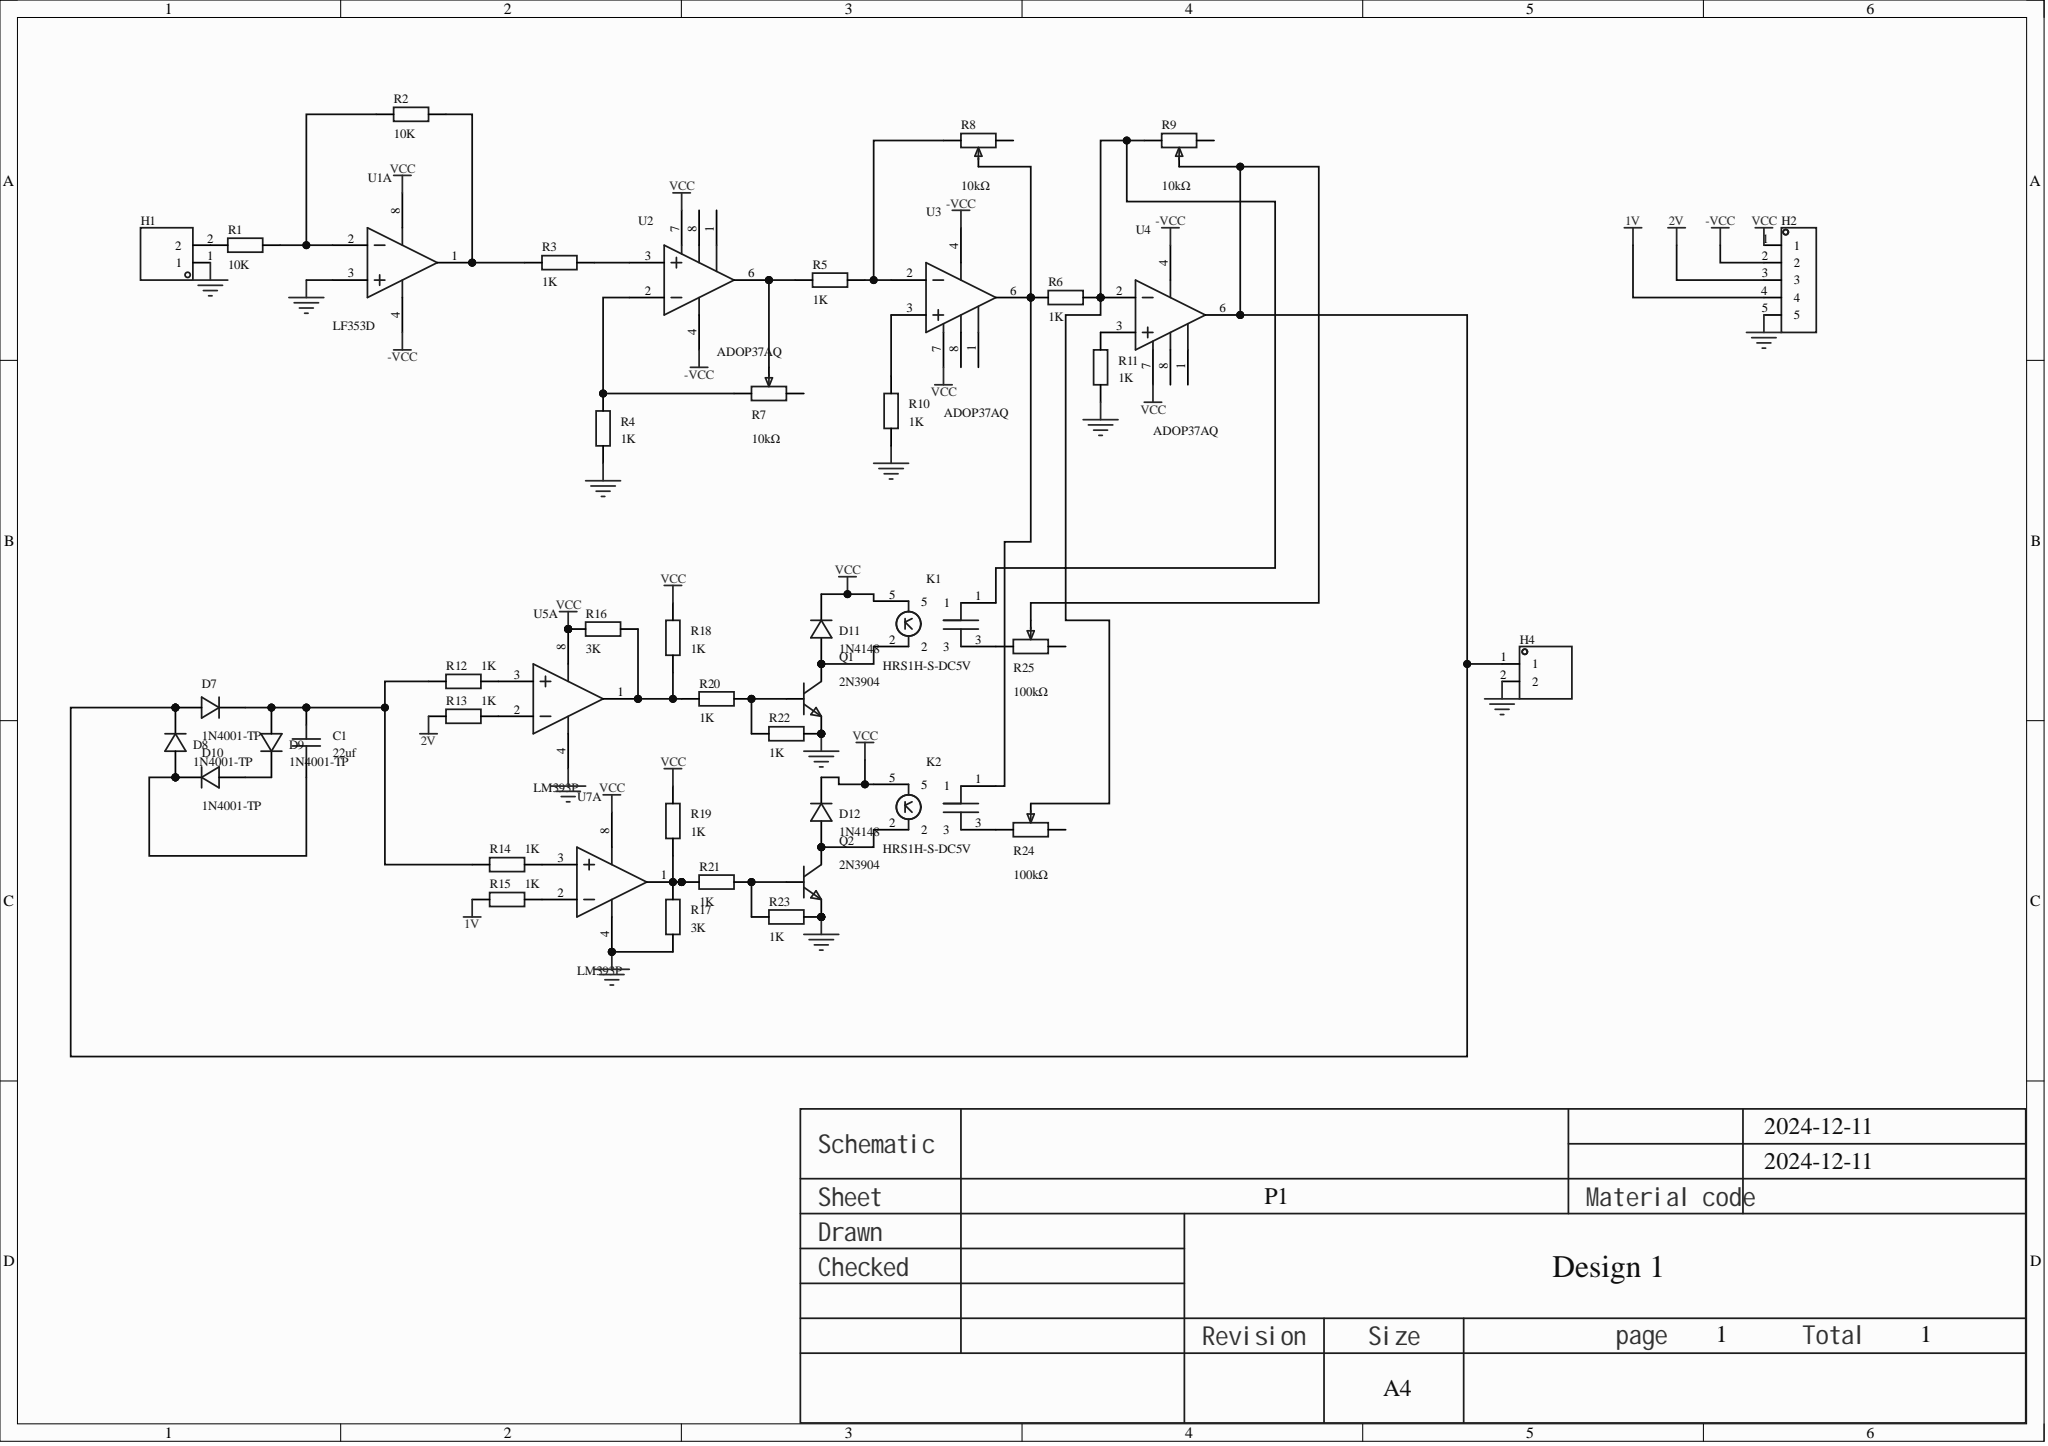Circuit board | Altium Designer | 45 parts | 32 nets
Bill of materials:
Comment,Description,Designator,Footprint,LibRef,Quantity
"22uf","","C1","C0805","CAP_0805","1"
"1N4001-TP","","D7, D8, D9, D10","DO-41_BD2.4-L4.7-P8.70-D0.9-RD","1N4001-TP","4"
"1N4148","Diode configuration: -; forward voltage (Vf): 1.1V@1A; DC reverse withstand voltage (Vr): 50V; rectified current: 1A;","D11, D12","DO-41_BD2.4-L4.7-P8.70-D0.9-RD","1N4001_C2456","2"
"","","H1, H4","HDR-TH_2P-P2.54-V-M-1","HDR-M_2.54_1x2P","2"
"","","H2","HDR-TH_5P-P2.54-V-M","HDR-M_2.54_1x5P","1"
"HRS1H-S-DC5V","Ultra-miniature relay 15.6x10.6x11.8 (mm), 3A contact switching capacity, single-pole changeover, high sensitivity","K1, K2","RELAY-TH_HRS1H-S-DC3V","HRS1H-S-DC5V","2"
"2N3904","Transistor type: NPN; collector current (Ic): 200mA; collector-emitter breakdown voltage (Vceo): 40V; power (Pd): 625mW; DC current gain (hFE@Ic,Vce): 60@50mA,1V;","Q1, Q2","TO-92-3_L4.9-W3.7-P1.27-L","2N3904","2"
"10K","","R1, R2","R0603","Res_0603","2"
"1K","","R3, R4, R5, R6, R10, R11, R12, R13, R14, R15, R18, R19, R20, R21, R22, R23","R0603","Res_0603","16"
"10kΩ","","R7, R8, R9","R_3296","R_3296","3"
"3K","","R16, R17","R0603","Res_0603","2"
"100kΩ","","R24, R25","R_3296","R_3296","2"
"LF353D","GBP: 3MHz; input bias current (Ib): 50pA; input offset voltage (Vos): 5mV; slew rate (SR): 13V/us;","U1","SOIC-8_L4.9-W3.9-P1.27-LS6.0-BL","LF353D","1"
"ADOP37AQ","Number of amplifiers: single; input bias current (Ib): 10nA; input offset voltage (Vos): 10uV; GBP: 63MHz; slew rate (SR): 17V/us; bandwidth (-3db): -;","U2, U3, U4","PDIP-8_L9.6-W6.4-P2.54-LS7.6-BL","ADOP37AQ","3"
"LM393P","Input offset voltage (Vos): 5mV; input bias current (Ib): 250nA;","U5, U7","DIP-8_L10.1-W6.3-P2.54-LS7.6-BL-1","LM393P","2"
Netlist (Protel format):
[
C1
C0805
22uf



]
[
D7
DO-41_BD2.4-L4.7-P8.70-D0.9-RD
1N4001-TP



]
[
D8
DO-41_BD2.4-L4.7-P8.70-D0.9-RD
1N4001-TP



]
[
D9
DO-41_BD2.4-L4.7-P8.70-D0.9-RD
1N4001-TP



]
[
D10
DO-41_BD2.4-L4.7-P8.70-D0.9-RD
1N4001-TP



]
[
D11
DO-41_BD2.4-L4.7-P8.70-D0.9-RD
1N4148



]
[
D12
DO-41_BD2.4-L4.7-P8.70-D0.9-RD
1N4148



]
[
H1
HDR-TH_2P-P2.54-V-M-1




]
[
H2
HDR-TH_5P-P2.54-V-M




]
[
H4
HDR-TH_2P-P2.54-V-M-1




]
[
K1
RELAY-TH_HRS1H-S-DC3V
HRS1H-S-DC5V



]
[
K2
RELAY-TH_HRS1H-S-DC3V
HRS1H-S-DC5V



]
[
Q1
TO-92-3_L4.9-W3.7-P1.27-L
2N3904



]
[
Q2
TO-92-3_L4.9-W3.7-P1.27-L
2N3904



]
[
R1
R0603
10K



]
[
R2
R0603
10K



]
[
R3
R0603
1K



]
[
R4
R0603
1K



]
[
R5
R0603
1K



]
[
R6
R0603
1K



]
[
R7
R_3296
10kΩ



]
[
R8
R_3296
10kΩ



]
[
R9
R_3296
10kΩ



]
[
R10
R0603
1K



]
[
R11
R0603
1K



]
[
R12
R0603
1K



]
[
R13
R0603
1K



]
[
R14
R0603
1K



]
[
R15
R0603
1K



]
[
R16
R0603
3K



]
[
R17
R0603
3K



]
[
R18
R0603
1K



]
[
R19
R0603
1K



]
[
R20
R0603
1K



]
[
R21
R0603
1K



]
[
R22
R0603
1K



]
[
R23
R0603
1K



]
[
R24
R_3296
100kΩ



]
[
R25
R_3296
100kΩ



]
[
U1
SOIC-8_L4.9-W3.9-P1.27-LS6.0-BL
LF353D



]
[
U2
PDIP-8_L9.6-W6.4-P2.54-LS7.6-BL
ADOP37AQ



]
[
U3
PDIP-8_L9.6-W6.4-P2.54-LS7.6-BL
ADOP37AQ



]
[
U4
PDIP-8_L9.6-W6.4-P2.54-LS7.6-BL
ADOP37AQ



]
[
U5
DIP-8_L10.1-W6.3-P2.54-LS7.6-BL-1
LM393P



]
[
U7
DIP-8_L10.1-W6.3-P2.54-LS7.6-BL-1
LM393P



]
(
VCC
D11-1
D12-1
H2-1
K1-5
K2-5
R16-1
R18-2
R19-2
U1-8
U2-7
U3-7
U4-7
U5-8
U7-8
)
(
NetR17_2
R17-2
R19-1
R21-1
U7-1
)
(
NetR16_2
R16-2
R18-1
R20-1
U5-1
)
(
NetR15_2
R15-2
U7-2
)
(
NetR14_2
R14-2
U7-3
)
(
NetR13_2
R13-2
U5-2
)
(
NetR12_2
R12-2
U5-3
)
(
NetR11_2
R11-2
U4-3
)
(
NetR10_2
R10-2
U3-3
)
(
NetR5_2
R5-2
R8-1
U3-2
)
(
NetR5_1
R5-1
R7-2
U2-6
)
(
NetR4_2
R4-2
R7-3
U2-2
)
(
NetR3_2
R3-2
U2-3
)
(
NetR2_2
R2-2
R3-1
U1-1
)
(
NetR1_2
R1-2
R2-1
U1-2
)
(
NetQ2_2
Q2-2
R21-2
R23-1
)
(
NetQ1_2
Q1-2
R20-2
R22-1
)
(
NetK2_3
K2-3
R24-3
)
(
NetK2_1
K2-1
R6-1
R8-2
U3-6
)
(
NetK1_3
K1-3
R25-3
)
(
NetK1_1
K1-1
R6-2
R9-1
R24-2
U4-2
)
(
NetH1_2
H1-2
R1-1
)
(
NetD12_2
D12-2
K2-2
Q2-3
)
(
NetD11_2
D11-2
K1-2
Q1-3
)
(
NetD9_1
D9-1
D10-2
)
(
NetD7_2
D7-2
D8-1
H4-1
R9-2
R25-2
U4-6
)
(
NetC1_2
C1-2
D7-1
D9-2
R12-1
R14-1
)
(
NetC1_1
C1-1
D8-2
D10-1
)
(
GND
H1-1
H2-5
H4-2
Q1-1
Q2-1
R4-1
R10-1
R11-1
R17-1
R22-2
R23-2
U1-3
U5-4
U7-4
)
(
-VCC
H2-2
U1-4
U2-4
U3-4
U4-4
)
(
2V
H2-3
R13-1
)
(
1V
H2-4
R15-1
)